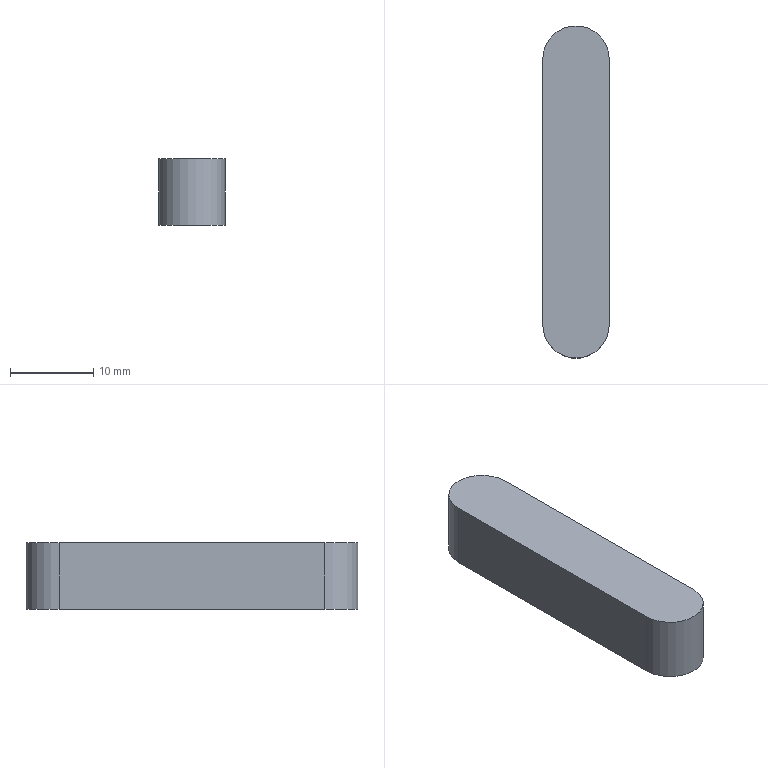Part | NX | features DATUM_CSYS 2, EXTRUDE 1, SKETCH 1 | 1 solid | 6 faces | box 8 x 40 x 8 mm | volume 2450 mm3 | plane 4 | cylinder 2 | commonest cylinder face diameters 8 x2
STEP:
#1=CARTESIAN_POINT('',(-4.,16.,0.));
#2=VERTEX_POINT('',#1);
#3=CARTESIAN_POINT('',(-4.,-16.,0.));
#4=VERTEX_POINT('',#3);
#5=CARTESIAN_POINT('',(-4.,16.,0.));
#6=DIRECTION('',(0.,-1.,0.));
#7=VECTOR('',#6,1000.);
#8=LINE('',#5,#7);
#9=EDGE_CURVE('',#2,#4,#8,.T.);
#10=ORIENTED_EDGE('',*,*,#9,.T.);
#11=CARTESIAN_POINT('',(-4.,-16.,8.));
#12=VERTEX_POINT('',#11);
#13=CARTESIAN_POINT('',(-4.,-16.,8.));
#14=DIRECTION('',(0.,0.,-1.));
#15=VECTOR('',#14,1000.);
#16=LINE('',#13,#15);
#17=EDGE_CURVE('',#12,#4,#16,.T.);
#18=ORIENTED_EDGE('',*,*,#17,.F.);
#19=CARTESIAN_POINT('',(-4.,16.,8.));
#20=VERTEX_POINT('',#19);
#21=CARTESIAN_POINT('',(-4.,16.,8.));
#22=DIRECTION('',(0.,-1.,0.));
#23=VECTOR('',#22,1000.);
#24=LINE('',#21,#23);
#25=EDGE_CURVE('',#20,#12,#24,.T.);
#26=ORIENTED_EDGE('',*,*,#25,.F.);
#27=CARTESIAN_POINT('',(-4.,16.,8.));
#28=DIRECTION('',(0.,0.,-1.));
#29=VECTOR('',#28,1000.);
#30=LINE('',#27,#29);
#31=EDGE_CURVE('',#20,#2,#30,.T.);
#32=ORIENTED_EDGE('',*,*,#31,.T.);
#33=EDGE_LOOP('',(#10,#18,#26,#32));
#34=FACE_BOUND('',#33,.T.);
#35=CARTESIAN_POINT('',(-4.,16.,8.));
#36=DIRECTION('',(1.,0.,0.));
#37=DIRECTION('',(0.,0.,-1.));
#38=AXIS2_PLACEMENT_3D('',#35,#36,#37);
#39=PLANE('',#38);
#40=ADVANCED_FACE('',(#34),#39,.F.);
#41=CARTESIAN_POINT('',(4.,-16.,0.));
#42=VERTEX_POINT('',#41);
#43=CARTESIAN_POINT('',(0.,-16.,0.));
#44=DIRECTION('',(0.,0.,1.));
#45=DIRECTION('',(1.,0.,0.));
#46=AXIS2_PLACEMENT_3D('',#43,#44,#45);
#47=CIRCLE('',#46,4.);
#48=EDGE_CURVE('',#4,#42,#47,.T.);
#49=ORIENTED_EDGE('',*,*,#48,.T.);
#50=CARTESIAN_POINT('',(4.,-16.,8.));
#51=VERTEX_POINT('',#50);
#52=CARTESIAN_POINT('',(4.,-16.,8.));
#53=DIRECTION('',(0.,0.,-1.));
#54=VECTOR('',#53,1000.);
#55=LINE('',#52,#54);
#56=EDGE_CURVE('',#51,#42,#55,.T.);
#57=ORIENTED_EDGE('',*,*,#56,.F.);
#58=CARTESIAN_POINT('',(0.,-16.,8.));
#59=DIRECTION('',(0.,0.,1.));
#60=DIRECTION('',(1.,0.,0.));
#61=AXIS2_PLACEMENT_3D('',#58,#59,#60);
#62=CIRCLE('',#61,4.);
#63=EDGE_CURVE('',#12,#51,#62,.T.);
#64=ORIENTED_EDGE('',*,*,#63,.F.);
#65=ORIENTED_EDGE('',*,*,#17,.T.);
#66=EDGE_LOOP('',(#49,#57,#64,#65));
#67=FACE_BOUND('',#66,.T.);
#68=CARTESIAN_POINT('',(0.,-16.,8.));
#69=DIRECTION('',(0.,0.,-1.));
#70=DIRECTION('',(-1.,0.,0.));
#71=AXIS2_PLACEMENT_3D('',#68,#69,#70);
#72=CYLINDRICAL_SURFACE('',#71,4.);
#73=ADVANCED_FACE('',(#67),#72,.T.);
#74=CARTESIAN_POINT('',(4.,16.,0.));
#75=VERTEX_POINT('',#74);
#76=CARTESIAN_POINT('',(4.,-16.,0.));
#77=DIRECTION('',(0.,1.,0.));
#78=VECTOR('',#77,1000.);
#79=LINE('',#76,#78);
#80=EDGE_CURVE('',#42,#75,#79,.T.);
#81=ORIENTED_EDGE('',*,*,#80,.T.);
#82=CARTESIAN_POINT('',(4.,16.,8.));
#83=VERTEX_POINT('',#82);
#84=CARTESIAN_POINT('',(4.,16.,8.));
#85=DIRECTION('',(0.,0.,-1.));
#86=VECTOR('',#85,1000.);
#87=LINE('',#84,#86);
#88=EDGE_CURVE('',#83,#75,#87,.T.);
#89=ORIENTED_EDGE('',*,*,#88,.F.);
#90=CARTESIAN_POINT('',(4.,-16.,8.));
#91=DIRECTION('',(0.,1.,0.));
#92=VECTOR('',#91,1000.);
#93=LINE('',#90,#92);
#94=EDGE_CURVE('',#51,#83,#93,.T.);
#95=ORIENTED_EDGE('',*,*,#94,.F.);
#96=ORIENTED_EDGE('',*,*,#56,.T.);
#97=EDGE_LOOP('',(#81,#89,#95,#96));
#98=FACE_BOUND('',#97,.T.);
#99=CARTESIAN_POINT('',(4.,-16.,8.));
#100=DIRECTION('',(-1.,0.,0.));
#101=DIRECTION('',(0.,0.,1.));
#102=AXIS2_PLACEMENT_3D('',#99,#100,#101);
#103=PLANE('',#102);
#104=ADVANCED_FACE('',(#98),#103,.F.);
#105=CARTESIAN_POINT('',(0.,16.,0.));
#106=DIRECTION('',(0.,0.,1.));
#107=DIRECTION('',(1.,0.,0.));
#108=AXIS2_PLACEMENT_3D('',#105,#106,#107);
#109=CIRCLE('',#108,4.);
#110=EDGE_CURVE('',#75,#2,#109,.T.);
#111=ORIENTED_EDGE('',*,*,#110,.T.);
#112=ORIENTED_EDGE('',*,*,#31,.F.);
#113=CARTESIAN_POINT('',(0.,16.,8.));
#114=DIRECTION('',(0.,0.,1.));
#115=DIRECTION('',(1.,0.,0.));
#116=AXIS2_PLACEMENT_3D('',#113,#114,#115);
#117=CIRCLE('',#116,4.);
#118=EDGE_CURVE('',#83,#20,#117,.T.);
#119=ORIENTED_EDGE('',*,*,#118,.F.);
#120=ORIENTED_EDGE('',*,*,#88,.T.);
#121=EDGE_LOOP('',(#111,#112,#119,#120));
#122=FACE_BOUND('',#121,.T.);
#123=CARTESIAN_POINT('',(0.,16.,8.));
#124=DIRECTION('',(0.,0.,-1.));
#125=DIRECTION('',(-1.,0.,0.));
#126=AXIS2_PLACEMENT_3D('',#123,#124,#125);
#127=CYLINDRICAL_SURFACE('',#126,4.);
#128=ADVANCED_FACE('',(#122),#127,.T.);
#129=ORIENTED_EDGE('',*,*,#25,.T.);
#130=ORIENTED_EDGE('',*,*,#63,.T.);
#131=ORIENTED_EDGE('',*,*,#94,.T.);
#132=ORIENTED_EDGE('',*,*,#118,.T.);
#133=EDGE_LOOP('',(#129,#130,#131,#132));
#134=FACE_BOUND('',#133,.T.);
#135=CARTESIAN_POINT('',(0.,-16.,8.));
#136=DIRECTION('',(0.,0.,1.));
#137=DIRECTION('',(1.,0.,0.));
#138=AXIS2_PLACEMENT_3D('',#135,#136,#137);
#139=PLANE('',#138);
#140=ADVANCED_FACE('',(#134),#139,.T.);
#141=ORIENTED_EDGE('',*,*,#9,.F.);
#142=ORIENTED_EDGE('',*,*,#110,.F.);
#143=ORIENTED_EDGE('',*,*,#80,.F.);
#144=ORIENTED_EDGE('',*,*,#48,.F.);
#145=EDGE_LOOP('',(#141,#142,#143,#144));
#146=FACE_BOUND('',#145,.T.);
#147=CARTESIAN_POINT('',(0.,-16.,0.));
#148=DIRECTION('',(0.,0.,1.));
#149=DIRECTION('',(1.,0.,0.));
#150=AXIS2_PLACEMENT_3D('',#147,#148,#149);
#151=PLANE('',#150);
#152=ADVANCED_FACE('',(#146),#151,.F.);
#153=CLOSED_SHELL('',(#40,#73,#104,#128,#140,#152));
#154=MANIFOLD_SOLID_BREP('',#153);
#155=(LENGTH_UNIT()NAMED_UNIT(*)SI_UNIT(.MILLI.,.METRE.));
#156=UNCERTAINTY_MEASURE_WITH_UNIT(LENGTH_MEASURE(0.00001),#155,'','');
#157=(NAMED_UNIT(*)PLANE_ANGLE_UNIT()SI_UNIT($,.RADIAN.));
#158=(NAMED_UNIT(*)SI_UNIT($,.STERADIAN.)SOLID_ANGLE_UNIT());
#159=(GEOMETRIC_REPRESENTATION_CONTEXT(3)GLOBAL_UNCERTAINTY_ASSIGNED_CONTEXT((#156))GLOBAL_UNIT_ASSIGNED_CONTEXT((#155,#157,#158))REPRESENTATION_CONTEXT('',''));
#160=ADVANCED_BREP_SHAPE_REPRESENTATION('',(#154),#159);